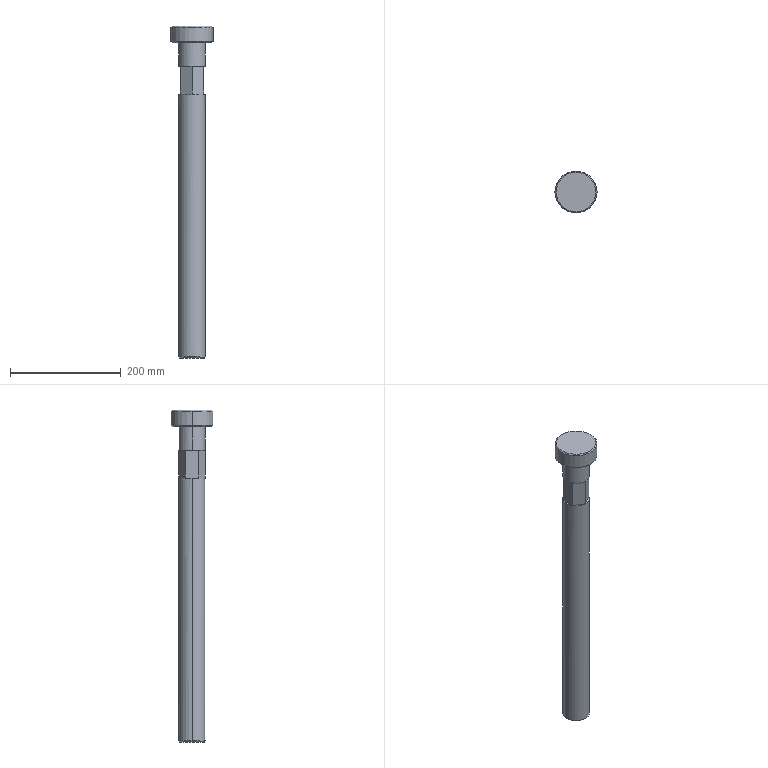Part | SolidWorks | features ICE 3, Chamfer 1, Extrusion 1 | 1 solid | 33 faces | box 76 x 76 x 600 mm | volume 1150657 mm3 | plane 21 | cone 6 | cylinder 6 | commonest cylinder face diameters 48 x4 76 x2
STEP:
#1=CARTESIAN_POINT('',(-22.,0.,-477.));
#2=VERTEX_POINT('',#1);
#3=CARTESIAN_POINT('',(22.,0.,-477.));
#4=VERTEX_POINT('',#3);
#5=CARTESIAN_POINT('',(0.,0.,-477.));
#6=DIRECTION('',(0.,0.,-1.));
#7=DIRECTION('',(-1.,0.,0.));
#8=AXIS2_PLACEMENT_3D('',#5,#6,#7);
#9=CIRCLE('',#8,22.);
#10=EDGE_CURVE('',#2,#4,#9,.T.);
#11=ORIENTED_EDGE('',*,*,#10,.F.);
#12=CARTESIAN_POINT('',(-24.,0.,-475.));
#13=VERTEX_POINT('',#12);
#14=CARTESIAN_POINT('',(-22.,0.,-477.));
#15=DIRECTION('',(-0.7071,0.,0.7071));
#16=VECTOR('',#15,1000.);
#17=LINE('',#14,#16);
#18=EDGE_CURVE('',#2,#13,#17,.T.);
#19=ORIENTED_EDGE('',*,*,#18,.T.);
#20=CARTESIAN_POINT('',(24.,0.,-475.));
#21=VERTEX_POINT('',#20);
#22=CARTESIAN_POINT('',(0.,0.,-475.));
#23=DIRECTION('',(0.,0.,1.));
#24=DIRECTION('',(-1.,0.,0.));
#25=AXIS2_PLACEMENT_3D('',#22,#23,#24);
#26=CIRCLE('',#25,24.);
#27=EDGE_CURVE('',#21,#13,#26,.T.);
#28=ORIENTED_EDGE('',*,*,#27,.F.);
#29=CARTESIAN_POINT('',(22.,0.,-477.));
#30=DIRECTION('',(0.7071,0.,0.7071));
#31=VECTOR('',#30,1000.);
#32=LINE('',#29,#31);
#33=EDGE_CURVE('',#4,#21,#32,.T.);
#34=ORIENTED_EDGE('',*,*,#33,.F.);
#35=EDGE_LOOP('',(#11,#19,#28,#34));
#36=FACE_OUTER_BOUND('',#35,.T.);
#37=CARTESIAN_POINT('',(0.,0.,-477.));
#38=DIRECTION('',(0.,0.,1.));
#39=DIRECTION('',(1.,0.,0.));
#40=AXIS2_PLACEMENT_3D('',#37,#38,#39);
#41=CONICAL_SURFACE('',#40,22.,0.7854);
#42=ADVANCED_FACE('',(#36),#41,.T.);
#43=CARTESIAN_POINT('',(36.,0.,123.));
#44=VERTEX_POINT('',#43);
#45=CARTESIAN_POINT('',(-36.,0.,123.));
#46=VERTEX_POINT('',#45);
#47=CARTESIAN_POINT('',(0.,0.,123.));
#48=DIRECTION('',(0.,0.,1.));
#49=DIRECTION('',(1.,0.,0.));
#50=AXIS2_PLACEMENT_3D('',#47,#48,#49);
#51=CIRCLE('',#50,36.);
#52=EDGE_CURVE('',#44,#46,#51,.T.);
#53=ORIENTED_EDGE('',*,*,#52,.F.);
#54=CARTESIAN_POINT('',(38.,0.,121.));
#55=VERTEX_POINT('',#54);
#56=CARTESIAN_POINT('',(36.,0.,123.));
#57=DIRECTION('',(0.7071,0.,-0.7071));
#58=VECTOR('',#57,1000.);
#59=LINE('',#56,#58);
#60=EDGE_CURVE('',#44,#55,#59,.T.);
#61=ORIENTED_EDGE('',*,*,#60,.T.);
#62=CARTESIAN_POINT('',(-38.,0.,121.));
#63=VERTEX_POINT('',#62);
#64=CARTESIAN_POINT('',(0.,0.,121.));
#65=DIRECTION('',(0.,0.,-1.));
#66=DIRECTION('',(1.,0.,0.));
#67=AXIS2_PLACEMENT_3D('',#64,#65,#66);
#68=CIRCLE('',#67,38.);
#69=EDGE_CURVE('',#63,#55,#68,.T.);
#70=ORIENTED_EDGE('',*,*,#69,.F.);
#71=CARTESIAN_POINT('',(-36.,0.,123.));
#72=DIRECTION('',(-0.7071,0.,-0.7071));
#73=VECTOR('',#72,1000.);
#74=LINE('',#71,#73);
#75=EDGE_CURVE('',#46,#63,#74,.T.);
#76=ORIENTED_EDGE('',*,*,#75,.F.);
#77=EDGE_LOOP('',(#53,#61,#70,#76));
#78=FACE_OUTER_BOUND('',#77,.T.);
#79=CARTESIAN_POINT('',(0.,0.,123.));
#80=DIRECTION('',(0.,0.,-1.));
#81=DIRECTION('',(-1.,0.,0.));
#82=AXIS2_PLACEMENT_3D('',#79,#80,#81);
#83=CONICAL_SURFACE('',#82,36.,0.7854);
#84=ADVANCED_FACE('',(#78),#83,.T.);
#85=CARTESIAN_POINT('',(-36.,0.,93.));
#86=VERTEX_POINT('',#85);
#87=CARTESIAN_POINT('',(36.,0.,93.));
#88=VERTEX_POINT('',#87);
#89=CARTESIAN_POINT('',(0.,0.,93.));
#90=DIRECTION('',(0.,0.,-1.));
#91=DIRECTION('',(1.,0.,0.));
#92=AXIS2_PLACEMENT_3D('',#89,#90,#91);
#93=CIRCLE('',#92,36.);
#94=EDGE_CURVE('',#86,#88,#93,.T.);
#95=ORIENTED_EDGE('',*,*,#94,.F.);
#96=CARTESIAN_POINT('',(-38.,0.,95.));
#97=VERTEX_POINT('',#96);
#98=CARTESIAN_POINT('',(-38.,0.,95.));
#99=DIRECTION('',(-0.7071,0.,0.7071));
#100=VECTOR('',#99,1000.);
#101=LINE('',#98,#100);
#102=EDGE_CURVE('',#86,#97,#101,.T.);
#103=ORIENTED_EDGE('',*,*,#102,.T.);
#104=CARTESIAN_POINT('',(38.,0.,95.));
#105=VERTEX_POINT('',#104);
#106=CARTESIAN_POINT('',(0.,0.,95.));
#107=DIRECTION('',(0.,0.,1.));
#108=DIRECTION('',(1.,0.,0.));
#109=AXIS2_PLACEMENT_3D('',#106,#107,#108);
#110=CIRCLE('',#109,38.);
#111=EDGE_CURVE('',#105,#97,#110,.T.);
#112=ORIENTED_EDGE('',*,*,#111,.F.);
#113=CARTESIAN_POINT('',(38.,0.,95.));
#114=DIRECTION('',(0.7071,0.,0.7071));
#115=VECTOR('',#114,1000.);
#116=LINE('',#113,#115);
#117=EDGE_CURVE('',#88,#105,#116,.T.);
#118=ORIENTED_EDGE('',*,*,#117,.F.);
#119=EDGE_LOOP('',(#95,#103,#112,#118));
#120=FACE_OUTER_BOUND('',#119,.T.);
#121=CARTESIAN_POINT('',(0.,0.,95.));
#122=DIRECTION('',(0.,0.,1.));
#123=DIRECTION('',(1.,0.,0.));
#124=AXIS2_PLACEMENT_3D('',#121,#122,#123);
#125=CONICAL_SURFACE('',#124,38.,0.7854);
#126=ADVANCED_FACE('',(#120),#125,.T.);
#127=ORIENTED_EDGE('',*,*,#27,.T.);
#128=CARTESIAN_POINT('',(-24.,0.,0.));
#129=VERTEX_POINT('',#128);
#130=CARTESIAN_POINT('',(-24.,0.,-477.));
#131=DIRECTION('',(0.,0.,1.));
#132=VECTOR('',#131,1000.);
#133=LINE('',#130,#132);
#134=EDGE_CURVE('',#13,#129,#133,.T.);
#135=ORIENTED_EDGE('',*,*,#134,.T.);
#136=CARTESIAN_POINT('',(-20.785,12.,0.));
#137=VERTEX_POINT('',#136);
#138=CARTESIAN_POINT('',(0.,0.,0.));
#139=DIRECTION('',(0.,0.,-1.));
#140=DIRECTION('',(-1.,0.,0.));
#141=AXIS2_PLACEMENT_3D('',#138,#139,#140);
#142=CIRCLE('',#141,24.);
#143=EDGE_CURVE('',#129,#137,#142,.T.);
#144=ORIENTED_EDGE('',*,*,#143,.T.);
#145=CARTESIAN_POINT('',(0.,24.,0.));
#146=VERTEX_POINT('',#145);
#147=CARTESIAN_POINT('',(0.,0.,0.));
#148=DIRECTION('',(0.,0.,-1.));
#149=DIRECTION('',(-1.,0.,0.));
#150=AXIS2_PLACEMENT_3D('',#147,#148,#149);
#151=CIRCLE('',#150,24.);
#152=EDGE_CURVE('',#137,#146,#151,.T.);
#153=ORIENTED_EDGE('',*,*,#152,.T.);
#154=CARTESIAN_POINT('',(20.785,12.,0.));
#155=VERTEX_POINT('',#154);
#156=CARTESIAN_POINT('',(0.,0.,0.));
#157=DIRECTION('',(0.,0.,-1.));
#158=DIRECTION('',(-1.,0.,0.));
#159=AXIS2_PLACEMENT_3D('',#156,#157,#158);
#160=CIRCLE('',#159,24.);
#161=EDGE_CURVE('',#146,#155,#160,.T.);
#162=ORIENTED_EDGE('',*,*,#161,.T.);
#163=CARTESIAN_POINT('',(24.,0.,0.));
#164=VERTEX_POINT('',#163);
#165=CARTESIAN_POINT('',(0.,0.,0.));
#166=DIRECTION('',(0.,0.,-1.));
#167=DIRECTION('',(-1.,0.,0.));
#168=AXIS2_PLACEMENT_3D('',#165,#166,#167);
#169=CIRCLE('',#168,24.);
#170=EDGE_CURVE('',#155,#164,#169,.T.);
#171=ORIENTED_EDGE('',*,*,#170,.T.);
#172=CARTESIAN_POINT('',(24.,0.,-477.));
#173=DIRECTION('',(0.,0.,1.));
#174=VECTOR('',#173,1000.);
#175=LINE('',#172,#174);
#176=EDGE_CURVE('',#21,#164,#175,.T.);
#177=ORIENTED_EDGE('',*,*,#176,.F.);
#178=EDGE_LOOP('',(#127,#135,#144,#153,#162,#171,#177));
#179=FACE_OUTER_BOUND('',#178,.T.);
#180=CARTESIAN_POINT('',(0.,0.,-477.));
#181=DIRECTION('',(0.,0.,1.));
#182=DIRECTION('',(1.,0.,0.));
#183=AXIS2_PLACEMENT_3D('',#180,#181,#182);
#184=CYLINDRICAL_SURFACE('',#183,24.);
#185=ADVANCED_FACE('',(#179),#184,.T.);
#186=ORIENTED_EDGE('',*,*,#69,.T.);
#187=CARTESIAN_POINT('',(38.,0.,123.));
#188=DIRECTION('',(0.,0.,-1.));
#189=VECTOR('',#188,1000.);
#190=LINE('',#187,#189);
#191=EDGE_CURVE('',#55,#105,#190,.T.);
#192=ORIENTED_EDGE('',*,*,#191,.T.);
#193=ORIENTED_EDGE('',*,*,#111,.T.);
#194=CARTESIAN_POINT('',(-38.,0.,123.));
#195=DIRECTION('',(0.,0.,-1.));
#196=VECTOR('',#195,1000.);
#197=LINE('',#194,#196);
#198=EDGE_CURVE('',#63,#97,#197,.T.);
#199=ORIENTED_EDGE('',*,*,#198,.F.);
#200=EDGE_LOOP('',(#186,#192,#193,#199));
#201=FACE_OUTER_BOUND('',#200,.T.);
#202=CARTESIAN_POINT('',(0.,0.,123.));
#203=DIRECTION('',(0.,0.,-1.));
#204=DIRECTION('',(-1.,0.,0.));
#205=AXIS2_PLACEMENT_3D('',#202,#203,#204);
#206=CYLINDRICAL_SURFACE('',#205,38.);
#207=ADVANCED_FACE('',(#201),#206,.T.);
#208=CARTESIAN_POINT('',(24.,0.,93.));
#209=VERTEX_POINT('',#208);
#210=CARTESIAN_POINT('',(-24.,0.,93.));
#211=VERTEX_POINT('',#210);
#212=CARTESIAN_POINT('',(0.,0.,93.));
#213=DIRECTION('',(0.,0.,1.));
#214=DIRECTION('',(1.,0.,0.));
#215=AXIS2_PLACEMENT_3D('',#212,#213,#214);
#216=CIRCLE('',#215,24.);
#217=EDGE_CURVE('',#209,#211,#216,.T.);
#218=ORIENTED_EDGE('',*,*,#217,.F.);
#219=CARTESIAN_POINT('',(24.,0.,50.));
#220=VERTEX_POINT('',#219);
#221=CARTESIAN_POINT('',(24.,0.,93.));
#222=DIRECTION('',(0.,0.,-1.));
#223=VECTOR('',#222,1000.);
#224=LINE('',#221,#223);
#225=EDGE_CURVE('',#209,#220,#224,.T.);
#226=ORIENTED_EDGE('',*,*,#225,.T.);
#227=CARTESIAN_POINT('',(20.785,12.,50.));
#228=VERTEX_POINT('',#227);
#229=CARTESIAN_POINT('',(0.,0.,50.));
#230=DIRECTION('',(0.,0.,1.));
#231=DIRECTION('',(1.,0.,0.));
#232=AXIS2_PLACEMENT_3D('',#229,#230,#231);
#233=CIRCLE('',#232,24.);
#234=EDGE_CURVE('',#220,#228,#233,.T.);
#235=ORIENTED_EDGE('',*,*,#234,.T.);
#236=CARTESIAN_POINT('',(0.,24.,50.));
#237=VERTEX_POINT('',#236);
#238=CARTESIAN_POINT('',(0.,0.,50.));
#239=DIRECTION('',(0.,0.,1.));
#240=DIRECTION('',(1.,0.,0.));
#241=AXIS2_PLACEMENT_3D('',#238,#239,#240);
#242=CIRCLE('',#241,24.);
#243=EDGE_CURVE('',#228,#237,#242,.T.);
#244=ORIENTED_EDGE('',*,*,#243,.T.);
#245=CARTESIAN_POINT('',(-20.785,12.,50.));
#246=VERTEX_POINT('',#245);
#247=CARTESIAN_POINT('',(0.,0.,50.));
#248=DIRECTION('',(0.,0.,1.));
#249=DIRECTION('',(1.,0.,0.));
#250=AXIS2_PLACEMENT_3D('',#247,#248,#249);
#251=CIRCLE('',#250,24.);
#252=EDGE_CURVE('',#237,#246,#251,.T.);
#253=ORIENTED_EDGE('',*,*,#252,.T.);
#254=CARTESIAN_POINT('',(-24.,0.,50.));
#255=VERTEX_POINT('',#254);
#256=CARTESIAN_POINT('',(0.,0.,50.));
#257=DIRECTION('',(0.,0.,1.));
#258=DIRECTION('',(1.,0.,0.));
#259=AXIS2_PLACEMENT_3D('',#256,#257,#258);
#260=CIRCLE('',#259,24.);
#261=EDGE_CURVE('',#246,#255,#260,.T.);
#262=ORIENTED_EDGE('',*,*,#261,.T.);
#263=CARTESIAN_POINT('',(-24.,0.,93.));
#264=DIRECTION('',(0.,0.,-1.));
#265=VECTOR('',#264,1000.);
#266=LINE('',#263,#265);
#267=EDGE_CURVE('',#211,#255,#266,.T.);
#268=ORIENTED_EDGE('',*,*,#267,.F.);
#269=EDGE_LOOP('',(#218,#226,#235,#244,#253,#262,#268));
#270=FACE_OUTER_BOUND('',#269,.T.);
#271=CARTESIAN_POINT('',(0.,0.,93.));
#272=DIRECTION('',(0.,0.,-1.));
#273=DIRECTION('',(-1.,0.,0.));
#274=AXIS2_PLACEMENT_3D('',#271,#272,#273);
#275=CYLINDRICAL_SURFACE('',#274,24.);
#276=ADVANCED_FACE('',(#270),#275,.T.);
#277=CARTESIAN_POINT('',(20.785,-12.,0.));
#278=VERTEX_POINT('',#277);
#279=CARTESIAN_POINT('',(20.785,-12.,0.));
#280=DIRECTION('',(0.,1.,0.));
#281=VECTOR('',#280,1000.);
#282=LINE('',#279,#281);
#283=EDGE_CURVE('',#278,#155,#282,.T.);
#284=ORIENTED_EDGE('',*,*,#283,.T.);
#285=CARTESIAN_POINT('',(20.785,12.,50.));
#286=DIRECTION('',(0.,0.,-1.));
#287=VECTOR('',#286,1000.);
#288=LINE('',#285,#287);
#289=EDGE_CURVE('',#228,#155,#288,.T.);
#290=ORIENTED_EDGE('',*,*,#289,.F.);
#291=CARTESIAN_POINT('',(20.785,-12.,50.));
#292=VERTEX_POINT('',#291);
#293=CARTESIAN_POINT('',(20.785,-12.,50.));
#294=DIRECTION('',(0.,1.,0.));
#295=VECTOR('',#294,1000.);
#296=LINE('',#293,#295);
#297=EDGE_CURVE('',#292,#228,#296,.T.);
#298=ORIENTED_EDGE('',*,*,#297,.F.);
#299=CARTESIAN_POINT('',(20.785,-12.,50.));
#300=DIRECTION('',(0.,0.,-1.));
#301=VECTOR('',#300,1000.);
#302=LINE('',#299,#301);
#303=EDGE_CURVE('',#292,#278,#302,.T.);
#304=ORIENTED_EDGE('',*,*,#303,.T.);
#305=EDGE_LOOP('',(#284,#290,#298,#304));
#306=FACE_OUTER_BOUND('',#305,.T.);
#307=CARTESIAN_POINT('',(20.785,-12.,50.));
#308=DIRECTION('',(-1.,0.,0.));
#309=DIRECTION('',(0.,-1.,0.));
#310=AXIS2_PLACEMENT_3D('',#307,#308,#309);
#311=PLANE('',#310);
#312=ADVANCED_FACE('',(#306),#311,.F.);
#313=CARTESIAN_POINT('',(20.785,12.,0.));
#314=DIRECTION('',(-0.866,0.5,0.));
#315=VECTOR('',#314,1000.);
#316=LINE('',#313,#315);
#317=EDGE_CURVE('',#155,#146,#316,.T.);
#318=ORIENTED_EDGE('',*,*,#317,.T.);
#319=CARTESIAN_POINT('',(0.,24.,50.));
#320=DIRECTION('',(0.,0.,-1.));
#321=VECTOR('',#320,1000.);
#322=LINE('',#319,#321);
#323=EDGE_CURVE('',#237,#146,#322,.T.);
#324=ORIENTED_EDGE('',*,*,#323,.F.);
#325=CARTESIAN_POINT('',(20.785,12.,50.));
#326=DIRECTION('',(-0.866,0.5,0.));
#327=VECTOR('',#326,1000.);
#328=LINE('',#325,#327);
#329=EDGE_CURVE('',#228,#237,#328,.T.);
#330=ORIENTED_EDGE('',*,*,#329,.F.);
#331=ORIENTED_EDGE('',*,*,#289,.T.);
#332=EDGE_LOOP('',(#318,#324,#330,#331));
#333=FACE_OUTER_BOUND('',#332,.T.);
#334=CARTESIAN_POINT('',(20.785,12.,50.));
#335=DIRECTION('',(-0.5,-0.866,0.));
#336=DIRECTION('',(0.866,-0.5,0.));
#337=AXIS2_PLACEMENT_3D('',#334,#335,#336);
#338=PLANE('',#337);
#339=ADVANCED_FACE('',(#333),#338,.F.);
#340=CARTESIAN_POINT('',(0.,24.,0.));
#341=DIRECTION('',(-0.866,-0.5,0.));
#342=VECTOR('',#341,1000.);
#343=LINE('',#340,#342);
#344=EDGE_CURVE('',#146,#137,#343,.T.);
#345=ORIENTED_EDGE('',*,*,#344,.T.);
#346=CARTESIAN_POINT('',(-20.785,12.,50.));
#347=DIRECTION('',(0.,0.,-1.));
#348=VECTOR('',#347,1000.);
#349=LINE('',#346,#348);
#350=EDGE_CURVE('',#246,#137,#349,.T.);
#351=ORIENTED_EDGE('',*,*,#350,.F.);
#352=CARTESIAN_POINT('',(0.,24.,50.));
#353=DIRECTION('',(-0.866,-0.5,0.));
#354=VECTOR('',#353,1000.);
#355=LINE('',#352,#354);
#356=EDGE_CURVE('',#237,#246,#355,.T.);
#357=ORIENTED_EDGE('',*,*,#356,.F.);
#358=ORIENTED_EDGE('',*,*,#323,.T.);
#359=EDGE_LOOP('',(#345,#351,#357,#358));
#360=FACE_OUTER_BOUND('',#359,.T.);
#361=CARTESIAN_POINT('',(0.,24.,50.));
#362=DIRECTION('',(0.5,-0.866,0.));
#363=DIRECTION('',(0.866,0.5,0.));
#364=AXIS2_PLACEMENT_3D('',#361,#362,#363);
#365=PLANE('',#364);
#366=ADVANCED_FACE('',(#360),#365,.F.);
#367=CARTESIAN_POINT('',(-20.785,-12.,0.));
#368=VERTEX_POINT('',#367);
#369=CARTESIAN_POINT('',(-20.785,12.,0.));
#370=DIRECTION('',(0.,-1.,0.));
#371=VECTOR('',#370,1000.);
#372=LINE('',#369,#371);
#373=EDGE_CURVE('',#137,#368,#372,.T.);
#374=ORIENTED_EDGE('',*,*,#373,.T.);
#375=CARTESIAN_POINT('',(-20.785,-12.,50.));
#376=VERTEX_POINT('',#375);
#377=CARTESIAN_POINT('',(-20.785,-12.,50.));
#378=DIRECTION('',(0.,0.,-1.));
#379=VECTOR('',#378,1000.);
#380=LINE('',#377,#379);
#381=EDGE_CURVE('',#376,#368,#380,.T.);
#382=ORIENTED_EDGE('',*,*,#381,.F.);
#383=CARTESIAN_POINT('',(-20.785,12.,50.));
#384=DIRECTION('',(0.,-1.,0.));
#385=VECTOR('',#384,1000.);
#386=LINE('',#383,#385);
#387=EDGE_CURVE('',#246,#376,#386,.T.);
#388=ORIENTED_EDGE('',*,*,#387,.F.);
#389=ORIENTED_EDGE('',*,*,#350,.T.);
#390=EDGE_LOOP('',(#374,#382,#388,#389));
#391=FACE_OUTER_BOUND('',#390,.T.);
#392=CARTESIAN_POINT('',(-20.785,12.,50.));
#393=DIRECTION('',(1.,0.,0.));
#394=DIRECTION('',(0.,1.,0.));
#395=AXIS2_PLACEMENT_3D('',#392,#393,#394);
#396=PLANE('',#395);
#397=ADVANCED_FACE('',(#391),#396,.F.);
#398=CARTESIAN_POINT('',(0.,-24.,0.));
#399=VERTEX_POINT('',#398);
#400=CARTESIAN_POINT('',(-20.785,-12.,0.));
#401=DIRECTION('',(0.866,-0.5,0.));
#402=VECTOR('',#401,1000.);
#403=LINE('',#400,#402);
#404=EDGE_CURVE('',#368,#399,#403,.T.);
#405=ORIENTED_EDGE('',*,*,#404,.T.);
#406=CARTESIAN_POINT('',(0.,-24.,50.));
#407=VERTEX_POINT('',#406);
#408=CARTESIAN_POINT('',(0.,-24.,50.));
#409=DIRECTION('',(0.,0.,-1.));
#410=VECTOR('',#409,1000.);
#411=LINE('',#408,#410);
#412=EDGE_CURVE('',#407,#399,#411,.T.);
#413=ORIENTED_EDGE('',*,*,#412,.F.);
#414=CARTESIAN_POINT('',(-20.785,-12.,50.));
#415=DIRECTION('',(0.866,-0.5,0.));
#416=VECTOR('',#415,1000.);
#417=LINE('',#414,#416);
#418=EDGE_CURVE('',#376,#407,#417,.T.);
#419=ORIENTED_EDGE('',*,*,#418,.F.);
#420=ORIENTED_EDGE('',*,*,#381,.T.);
#421=EDGE_LOOP('',(#405,#413,#419,#420));
#422=FACE_OUTER_BOUND('',#421,.T.);
#423=CARTESIAN_POINT('',(-20.785,-12.,50.));
#424=DIRECTION('',(0.5,0.866,0.));
#425=DIRECTION('',(-0.866,0.5,0.));
#426=AXIS2_PLACEMENT_3D('',#423,#424,#425);
#427=PLANE('',#426);
#428=ADVANCED_FACE('',(#422),#427,.F.);
#429=CARTESIAN_POINT('',(0.,-24.,0.));
#430=DIRECTION('',(0.866,0.5,0.));
#431=VECTOR('',#430,1000.);
#432=LINE('',#429,#431);
#433=EDGE_CURVE('',#399,#278,#432,.T.);
#434=ORIENTED_EDGE('',*,*,#433,.T.);
#435=ORIENTED_EDGE('',*,*,#303,.F.);
#436=CARTESIAN_POINT('',(0.,-24.,50.));
#437=DIRECTION('',(0.866,0.5,0.));
#438=VECTOR('',#437,1000.);
#439=LINE('',#436,#438);
#440=EDGE_CURVE('',#407,#292,#439,.T.);
#441=ORIENTED_EDGE('',*,*,#440,.F.);
#442=ORIENTED_EDGE('',*,*,#412,.T.);
#443=EDGE_LOOP('',(#434,#435,#441,#442));
#444=FACE_OUTER_BOUND('',#443,.T.);
#445=CARTESIAN_POINT('',(0.,-24.,50.));
#446=DIRECTION('',(-0.5,0.866,0.));
#447=DIRECTION('',(-0.866,-0.5,0.));
#448=AXIS2_PLACEMENT_3D('',#445,#446,#447);
#449=PLANE('',#448);
#450=ADVANCED_FACE('',(#444),#449,.F.);
#451=CARTESIAN_POINT('',(0.,0.,50.));
#452=DIRECTION('',(0.,0.,1.));
#453=DIRECTION('',(1.,0.,0.));
#454=AXIS2_PLACEMENT_3D('',#451,#452,#453);
#455=CIRCLE('',#454,24.);
#456=EDGE_CURVE('',#292,#220,#455,.T.);
#457=ORIENTED_EDGE('',*,*,#456,.F.);
#458=ORIENTED_EDGE('',*,*,#297,.T.);
#459=ORIENTED_EDGE('',*,*,#234,.F.);
#460=EDGE_LOOP('',(#457,#458,#459));
#461=FACE_OUTER_BOUND('',#460,.T.);
#462=CARTESIAN_POINT('',(0.,0.,50.));
#463=DIRECTION('',(0.,0.,1.));
#464=DIRECTION('',(1.,0.,0.));
#465=AXIS2_PLACEMENT_3D('',#462,#463,#464);
#466=PLANE('',#465);
#467=ADVANCED_FACE('',(#461),#466,.F.);
#468=ORIENTED_EDGE('',*,*,#243,.F.);
#469=ORIENTED_EDGE('',*,*,#329,.T.);
#470=EDGE_LOOP('',(#468,#469));
#471=FACE_OUTER_BOUND('',#470,.T.);
#472=CARTESIAN_POINT('',(0.,0.,50.));
#473=DIRECTION('',(0.,0.,1.));
#474=DIRECTION('',(1.,0.,0.));
#475=AXIS2_PLACEMENT_3D('',#472,#473,#474);
#476=PLANE('',#475);
#477=ADVANCED_FACE('',(#471),#476,.F.);
#478=ORIENTED_EDGE('',*,*,#252,.F.);
#479=ORIENTED_EDGE('',*,*,#356,.T.);
#480=EDGE_LOOP('',(#478,#479));
#481=FACE_OUTER_BOUND('',#480,.T.);
#482=CARTESIAN_POINT('',(0.,0.,50.));
#483=DIRECTION('',(0.,0.,1.));
#484=DIRECTION('',(1.,0.,0.));
#485=AXIS2_PLACEMENT_3D('',#482,#483,#484);
#486=PLANE('',#485);
#487=ADVANCED_FACE('',(#481),#486,.F.);
#488=ORIENTED_EDGE('',*,*,#261,.F.);
#489=ORIENTED_EDGE('',*,*,#387,.T.);
#490=CARTESIAN_POINT('',(0.,0.,50.));
#491=DIRECTION('',(0.,0.,1.));
#492=DIRECTION('',(1.,0.,0.));
#493=AXIS2_PLACEMENT_3D('',#490,#491,#492);
#494=CIRCLE('',#493,24.);
#495=EDGE_CURVE('',#255,#376,#494,.T.);
#496=ORIENTED_EDGE('',*,*,#495,.F.);
#497=EDGE_LOOP('',(#488,#489,#496));
#498=FACE_OUTER_BOUND('',#497,.T.);
#499=CARTESIAN_POINT('',(0.,0.,50.));
#500=DIRECTION('',(0.,0.,1.));
#501=DIRECTION('',(1.,0.,0.));
#502=AXIS2_PLACEMENT_3D('',#499,#500,#501);
#503=PLANE('',#502);
#504=ADVANCED_FACE('',(#498),#503,.F.);
#505=CARTESIAN_POINT('',(0.,0.,50.));
#506=DIRECTION('',(0.,0.,1.));
#507=DIRECTION('',(1.,0.,0.));
#508=AXIS2_PLACEMENT_3D('',#505,#506,#507);
#509=CIRCLE('',#508,24.);
#510=EDGE_CURVE('',#376,#407,#509,.T.);
#511=ORIENTED_EDGE('',*,*,#510,.F.);
#512=ORIENTED_EDGE('',*,*,#418,.T.);
#513=EDGE_LOOP('',(#511,#512));
#514=FACE_OUTER_BOUND('',#513,.T.);
#515=CARTESIAN_POINT('',(0.,0.,50.));
#516=DIRECTION('',(0.,0.,1.));
#517=DIRECTION('',(1.,0.,0.));
#518=AXIS2_PLACEMENT_3D('',#515,#516,#517);
#519=PLANE('',#518);
#520=ADVANCED_FACE('',(#514),#519,.F.);
#521=ORIENTED_EDGE('',*,*,#225,.F.);
#522=CARTESIAN_POINT('',(0.,0.,93.));
#523=DIRECTION('',(0.,0.,1.));
#524=DIRECTION('',(1.,0.,0.));
#525=AXIS2_PLACEMENT_3D('',#522,#523,#524);
#526=CIRCLE('',#525,24.);
#527=EDGE_CURVE('',#211,#209,#526,.T.);
#528=ORIENTED_EDGE('',*,*,#527,.F.);
#529=ORIENTED_EDGE('',*,*,#267,.T.);
#530=ORIENTED_EDGE('',*,*,#495,.T.);
#531=ORIENTED_EDGE('',*,*,#510,.T.);
#532=CARTESIAN_POINT('',(0.,0.,50.));
#533=DIRECTION('',(0.,0.,1.));
#534=DIRECTION('',(1.,0.,0.));
#535=AXIS2_PLACEMENT_3D('',#532,#533,#534);
#536=CIRCLE('',#535,24.);
#537=EDGE_CURVE('',#407,#292,#536,.T.);
#538=ORIENTED_EDGE('',*,*,#537,.T.);
#539=ORIENTED_EDGE('',*,*,#456,.T.);
#540=EDGE_LOOP('',(#521,#528,#529,#530,#531,#538,#539));
#541=FACE_OUTER_BOUND('',#540,.T.);
#542=CARTESIAN_POINT('',(0.,0.,93.));
#543=DIRECTION('',(0.,0.,-1.));
#544=DIRECTION('',(-1.,0.,0.));
#545=AXIS2_PLACEMENT_3D('',#542,#543,#544);
#546=CYLINDRICAL_SURFACE('',#545,24.);
#547=ADVANCED_FACE('',(#541),#546,.T.);
#548=ORIENTED_EDGE('',*,*,#537,.F.);
#549=ORIENTED_EDGE('',*,*,#440,.T.);
#550=EDGE_LOOP('',(#548,#549));
#551=FACE_OUTER_BOUND('',#550,.T.);
#552=CARTESIAN_POINT('',(0.,0.,50.));
#553=DIRECTION('',(0.,0.,1.));
#554=DIRECTION('',(1.,0.,0.));
#555=AXIS2_PLACEMENT_3D('',#552,#553,#554);
#556=PLANE('',#555);
#557=ADVANCED_FACE('',(#551),#556,.F.);
#558=ORIENTED_EDGE('',*,*,#191,.F.);
#559=CARTESIAN_POINT('',(0.,0.,121.));
#560=DIRECTION('',(0.,0.,-1.));
#561=DIRECTION('',(1.,0.,0.));
#562=AXIS2_PLACEMENT_3D('',#559,#560,#561);
#563=CIRCLE('',#562,38.);
#564=EDGE_CURVE('',#55,#63,#563,.T.);
#565=ORIENTED_EDGE('',*,*,#564,.T.);
#566=ORIENTED_EDGE('',*,*,#198,.T.);
#567=CARTESIAN_POINT('',(0.,0.,95.));
#568=DIRECTION('',(0.,0.,1.));
#569=DIRECTION('',(1.,0.,0.));
#570=AXIS2_PLACEMENT_3D('',#567,#568,#569);
#571=CIRCLE('',#570,38.);
#572=EDGE_CURVE('',#97,#105,#571,.T.);
#573=ORIENTED_EDGE('',*,*,#572,.T.);
#574=EDGE_LOOP('',(#558,#565,#566,#573));
#575=FACE_OUTER_BOUND('',#574,.T.);
#576=CARTESIAN_POINT('',(0.,0.,123.));
#577=DIRECTION('',(0.,0.,-1.));
#578=DIRECTION('',(-1.,0.,0.));
#579=AXIS2_PLACEMENT_3D('',#576,#577,#578);
#580=CYLINDRICAL_SURFACE('',#579,38.);
#581=ADVANCED_FACE('',(#575),#580,.T.);
#582=CARTESIAN_POINT('',(0.,0.,123.));
#583=DIRECTION('',(0.,0.,1.));
#584=DIRECTION('',(1.,0.,0.));
#585=AXIS2_PLACEMENT_3D('',#582,#583,#584);
#586=CIRCLE('',#585,36.);
#587=EDGE_CURVE('',#46,#44,#586,.T.);
#588=ORIENTED_EDGE('',*,*,#587,.T.);
#589=ORIENTED_EDGE('',*,*,#52,.T.);
#590=EDGE_LOOP('',(#588,#589));
#591=FACE_OUTER_BOUND('',#590,.T.);
#592=CARTESIAN_POINT('',(0.,0.,123.));
#593=DIRECTION('',(0.,0.,1.));
#594=DIRECTION('',(1.,0.,0.));
#595=AXIS2_PLACEMENT_3D('',#592,#593,#594);
#596=PLANE('',#595);
#597=ADVANCED_FACE('',(#591),#596,.T.);
#598=CARTESIAN_POINT('',(0.,0.,93.));
#599=DIRECTION('',(0.,0.,-1.));
#600=DIRECTION('',(1.,0.,0.));
#601=AXIS2_PLACEMENT_3D('',#598,#599,#600);
#602=CIRCLE('',#601,36.);
#603=EDGE_CURVE('',#88,#86,#602,.T.);
#604=ORIENTED_EDGE('',*,*,#603,.T.);
#605=ORIENTED_EDGE('',*,*,#94,.T.);
#606=EDGE_LOOP('',(#604,#605));
#607=FACE_OUTER_BOUND('',#606,.T.);
#608=ORIENTED_EDGE('',*,*,#527,.T.);
#609=ORIENTED_EDGE('',*,*,#217,.T.);
#610=EDGE_LOOP('',(#608,#609));
#611=FACE_BOUND('',#610,.T.);
#612=CARTESIAN_POINT('',(0.,0.,93.));
#613=DIRECTION('',(0.,0.,1.));
#614=DIRECTION('',(1.,0.,0.));
#615=AXIS2_PLACEMENT_3D('',#612,#613,#614);
#616=PLANE('',#615);
#617=ADVANCED_FACE('',(#607,#611),#616,.F.);
#618=ORIENTED_EDGE('',*,*,#283,.F.);
#619=CARTESIAN_POINT('',(0.,0.,0.));
#620=DIRECTION('',(0.,0.,-1.));
#621=DIRECTION('',(-1.,0.,0.));
#622=AXIS2_PLACEMENT_3D('',#619,#620,#621);
#623=CIRCLE('',#622,24.);
#624=EDGE_CURVE('',#164,#278,#623,.T.);
#625=ORIENTED_EDGE('',*,*,#624,.F.);
#626=ORIENTED_EDGE('',*,*,#170,.F.);
#627=EDGE_LOOP('',(#618,#625,#626));
#628=FACE_OUTER_BOUND('',#627,.T.);
#629=CARTESIAN_POINT('',(0.,0.,0.));
#630=DIRECTION('',(0.,0.,-1.));
#631=DIRECTION('',(-1.,0.,0.));
#632=AXIS2_PLACEMENT_3D('',#629,#630,#631);
#633=PLANE('',#632);
#634=ADVANCED_FACE('',(#628),#633,.F.);
#635=ORIENTED_EDGE('',*,*,#433,.F.);
#636=CARTESIAN_POINT('',(0.,0.,0.));
#637=DIRECTION('',(0.,0.,-1.));
#638=DIRECTION('',(-1.,0.,0.));
#639=AXIS2_PLACEMENT_3D('',#636,#637,#638);
#640=CIRCLE('',#639,24.);
#641=EDGE_CURVE('',#278,#399,#640,.T.);
#642=ORIENTED_EDGE('',*,*,#641,.F.);
#643=EDGE_LOOP('',(#635,#642));
#644=FACE_OUTER_BOUND('',#643,.T.);
#645=CARTESIAN_POINT('',(0.,0.,0.));
#646=DIRECTION('',(0.,0.,-1.));
#647=DIRECTION('',(-1.,0.,0.));
#648=AXIS2_PLACEMENT_3D('',#645,#646,#647);
#649=PLANE('',#648);
#650=ADVANCED_FACE('',(#644),#649,.F.);
#651=ORIENTED_EDGE('',*,*,#404,.F.);
#652=CARTESIAN_POINT('',(0.,0.,0.));
#653=DIRECTION('',(0.,0.,-1.));
#654=DIRECTION('',(-1.,0.,0.));
#655=AXIS2_PLACEMENT_3D('',#652,#653,#654);
#656=CIRCLE('',#655,24.);
#657=EDGE_CURVE('',#399,#368,#656,.T.);
#658=ORIENTED_EDGE('',*,*,#657,.F.);
#659=EDGE_LOOP('',(#651,#658));
#660=FACE_OUTER_BOUND('',#659,.T.);
#661=CARTESIAN_POINT('',(0.,0.,0.));
#662=DIRECTION('',(0.,0.,-1.));
#663=DIRECTION('',(-1.,0.,0.));
#664=AXIS2_PLACEMENT_3D('',#661,#662,#663);
#665=PLANE('',#664);
#666=ADVANCED_FACE('',(#660),#665,.F.);
#667=ORIENTED_EDGE('',*,*,#373,.F.);
#668=ORIENTED_EDGE('',*,*,#143,.F.);
#669=CARTESIAN_POINT('',(0.,0.,0.));
#670=DIRECTION('',(0.,0.,-1.));
#671=DIRECTION('',(-1.,0.,0.));
#672=AXIS2_PLACEMENT_3D('',#669,#670,#671);
#673=CIRCLE('',#672,24.);
#674=EDGE_CURVE('',#368,#129,#673,.T.);
#675=ORIENTED_EDGE('',*,*,#674,.F.);
#676=EDGE_LOOP('',(#667,#668,#675));
#677=FACE_OUTER_BOUND('',#676,.T.);
#678=CARTESIAN_POINT('',(0.,0.,0.));
#679=DIRECTION('',(0.,0.,-1.));
#680=DIRECTION('',(-1.,0.,0.));
#681=AXIS2_PLACEMENT_3D('',#678,#679,#680);
#682=PLANE('',#681);
#683=ADVANCED_FACE('',(#677),#682,.F.);
#684=ORIENTED_EDGE('',*,*,#344,.F.);
#685=ORIENTED_EDGE('',*,*,#152,.F.);
#686=EDGE_LOOP('',(#684,#685));
#687=FACE_OUTER_BOUND('',#686,.T.);
#688=CARTESIAN_POINT('',(0.,0.,0.));
#689=DIRECTION('',(0.,0.,-1.));
#690=DIRECTION('',(-1.,0.,0.));
#691=AXIS2_PLACEMENT_3D('',#688,#689,#690);
#692=PLANE('',#691);
#693=ADVANCED_FACE('',(#687),#692,.F.);
#694=ORIENTED_EDGE('',*,*,#317,.F.);
#695=ORIENTED_EDGE('',*,*,#161,.F.);
#696=EDGE_LOOP('',(#694,#695));
#697=FACE_OUTER_BOUND('',#696,.T.);
#698=CARTESIAN_POINT('',(0.,0.,0.));
#699=DIRECTION('',(0.,0.,-1.));
#700=DIRECTION('',(-1.,0.,0.));
#701=AXIS2_PLACEMENT_3D('',#698,#699,#700);
#702=PLANE('',#701);
#703=ADVANCED_FACE('',(#697),#702,.F.);
#704=ORIENTED_EDGE('',*,*,#134,.F.);
#705=CARTESIAN_POINT('',(0.,0.,-475.));
#706=DIRECTION('',(0.,0.,1.));
#707=DIRECTION('',(-1.,0.,0.));
#708=AXIS2_PLACEMENT_3D('',#705,#706,#707);
#709=CIRCLE('',#708,24.);
#710=EDGE_CURVE('',#13,#21,#709,.T.);
#711=ORIENTED_EDGE('',*,*,#710,.T.);
#712=ORIENTED_EDGE('',*,*,#176,.T.);
#713=ORIENTED_EDGE('',*,*,#624,.T.);
#714=ORIENTED_EDGE('',*,*,#641,.T.);
#715=ORIENTED_EDGE('',*,*,#657,.T.);
#716=ORIENTED_EDGE('',*,*,#674,.T.);
#717=EDGE_LOOP('',(#704,#711,#712,#713,#714,#715,#716));
#718=FACE_OUTER_BOUND('',#717,.T.);
#719=CARTESIAN_POINT('',(0.,0.,-477.));
#720=DIRECTION('',(0.,0.,1.));
#721=DIRECTION('',(1.,0.,0.));
#722=AXIS2_PLACEMENT_3D('',#719,#720,#721);
#723=CYLINDRICAL_SURFACE('',#722,24.);
#724=ADVANCED_FACE('',(#718),#723,.T.);
#725=CARTESIAN_POINT('',(0.,0.,-477.));
#726=DIRECTION('',(0.,0.,-1.));
#727=DIRECTION('',(-1.,0.,0.));
#728=AXIS2_PLACEMENT_3D('',#725,#726,#727);
#729=CIRCLE('',#728,22.);
#730=EDGE_CURVE('',#4,#2,#729,.T.);
#731=ORIENTED_EDGE('',*,*,#730,.T.);
#732=ORIENTED_EDGE('',*,*,#10,.T.);
#733=EDGE_LOOP('',(#731,#732));
#734=FACE_OUTER_BOUND('',#733,.T.);
#735=CARTESIAN_POINT('',(0.,0.,-477.));
#736=DIRECTION('',(0.,0.,-1.));
#737=DIRECTION('',(-1.,0.,0.));
#738=AXIS2_PLACEMENT_3D('',#735,#736,#737);
#739=PLANE('',#738);
#740=ADVANCED_FACE('',(#734),#739,.T.);
#741=ORIENTED_EDGE('',*,*,#102,.F.);
#742=ORIENTED_EDGE('',*,*,#603,.F.);
#743=ORIENTED_EDGE('',*,*,#117,.T.);
#744=ORIENTED_EDGE('',*,*,#572,.F.);
#745=EDGE_LOOP('',(#741,#742,#743,#744));
#746=FACE_OUTER_BOUND('',#745,.T.);
#747=CARTESIAN_POINT('',(0.,0.,95.));
#748=DIRECTION('',(0.,0.,1.));
#749=DIRECTION('',(1.,0.,0.));
#750=AXIS2_PLACEMENT_3D('',#747,#748,#749);
#751=CONICAL_SURFACE('',#750,38.,0.7854);
#752=ADVANCED_FACE('',(#746),#751,.T.);
#753=ORIENTED_EDGE('',*,*,#60,.F.);
#754=ORIENTED_EDGE('',*,*,#587,.F.);
#755=ORIENTED_EDGE('',*,*,#75,.T.);
#756=ORIENTED_EDGE('',*,*,#564,.F.);
#757=EDGE_LOOP('',(#753,#754,#755,#756));
#758=FACE_OUTER_BOUND('',#757,.T.);
#759=CARTESIAN_POINT('',(0.,0.,123.));
#760=DIRECTION('',(0.,0.,-1.));
#761=DIRECTION('',(-1.,0.,0.));
#762=AXIS2_PLACEMENT_3D('',#759,#760,#761);
#763=CONICAL_SURFACE('',#762,36.,0.7854);
#764=ADVANCED_FACE('',(#758),#763,.T.);
#765=ORIENTED_EDGE('',*,*,#18,.F.);
#766=ORIENTED_EDGE('',*,*,#730,.F.);
#767=ORIENTED_EDGE('',*,*,#33,.T.);
#768=ORIENTED_EDGE('',*,*,#710,.F.);
#769=EDGE_LOOP('',(#765,#766,#767,#768));
#770=FACE_OUTER_BOUND('',#769,.T.);
#771=CARTESIAN_POINT('',(0.,0.,-477.));
#772=DIRECTION('',(0.,0.,1.));
#773=DIRECTION('',(1.,0.,0.));
#774=AXIS2_PLACEMENT_3D('',#771,#772,#773);
#775=CONICAL_SURFACE('',#774,22.,0.7854);
#776=ADVANCED_FACE('',(#770),#775,.T.);
#777=CLOSED_SHELL('',(#42,#84,#126,#185,#207,#276,#312,#339,#366,#397,#428,#450,#467,#477,#487,#504,#520,#547,#557,#581,#597,#617,#634,#650,#666,#683,#693,#703,#724,#740,#752,#764,#776));
#778=MANIFOLD_SOLID_BREP('',#777);
#779=CARTESIAN_POINT('',(0.,0.,0.));
#780=DIRECTION('',(0.,0.,1.));
#781=DIRECTION('',(1.,0.,0.));
#782=AXIS2_PLACEMENT_3D('',#779,#780,#781);
#783=(LENGTH_UNIT()NAMED_UNIT(*)SI_UNIT(.MILLI.,.METRE.));
#784=UNCERTAINTY_MEASURE_WITH_UNIT(LENGTH_MEASURE(0.00001),#783,'','');
#785=(NAMED_UNIT(*)PLANE_ANGLE_UNIT()SI_UNIT($,.RADIAN.));
#786=(NAMED_UNIT(*)SI_UNIT($,.STERADIAN.)SOLID_ANGLE_UNIT());
#787=(GEOMETRIC_REPRESENTATION_CONTEXT(3)GLOBAL_UNCERTAINTY_ASSIGNED_CONTEXT((#784))GLOBAL_UNIT_ASSIGNED_CONTEXT((#783,#785,#786))REPRESENTATION_CONTEXT('',''));
#788=ADVANCED_BREP_SHAPE_REPRESENTATION('',(#778,#782),#787);